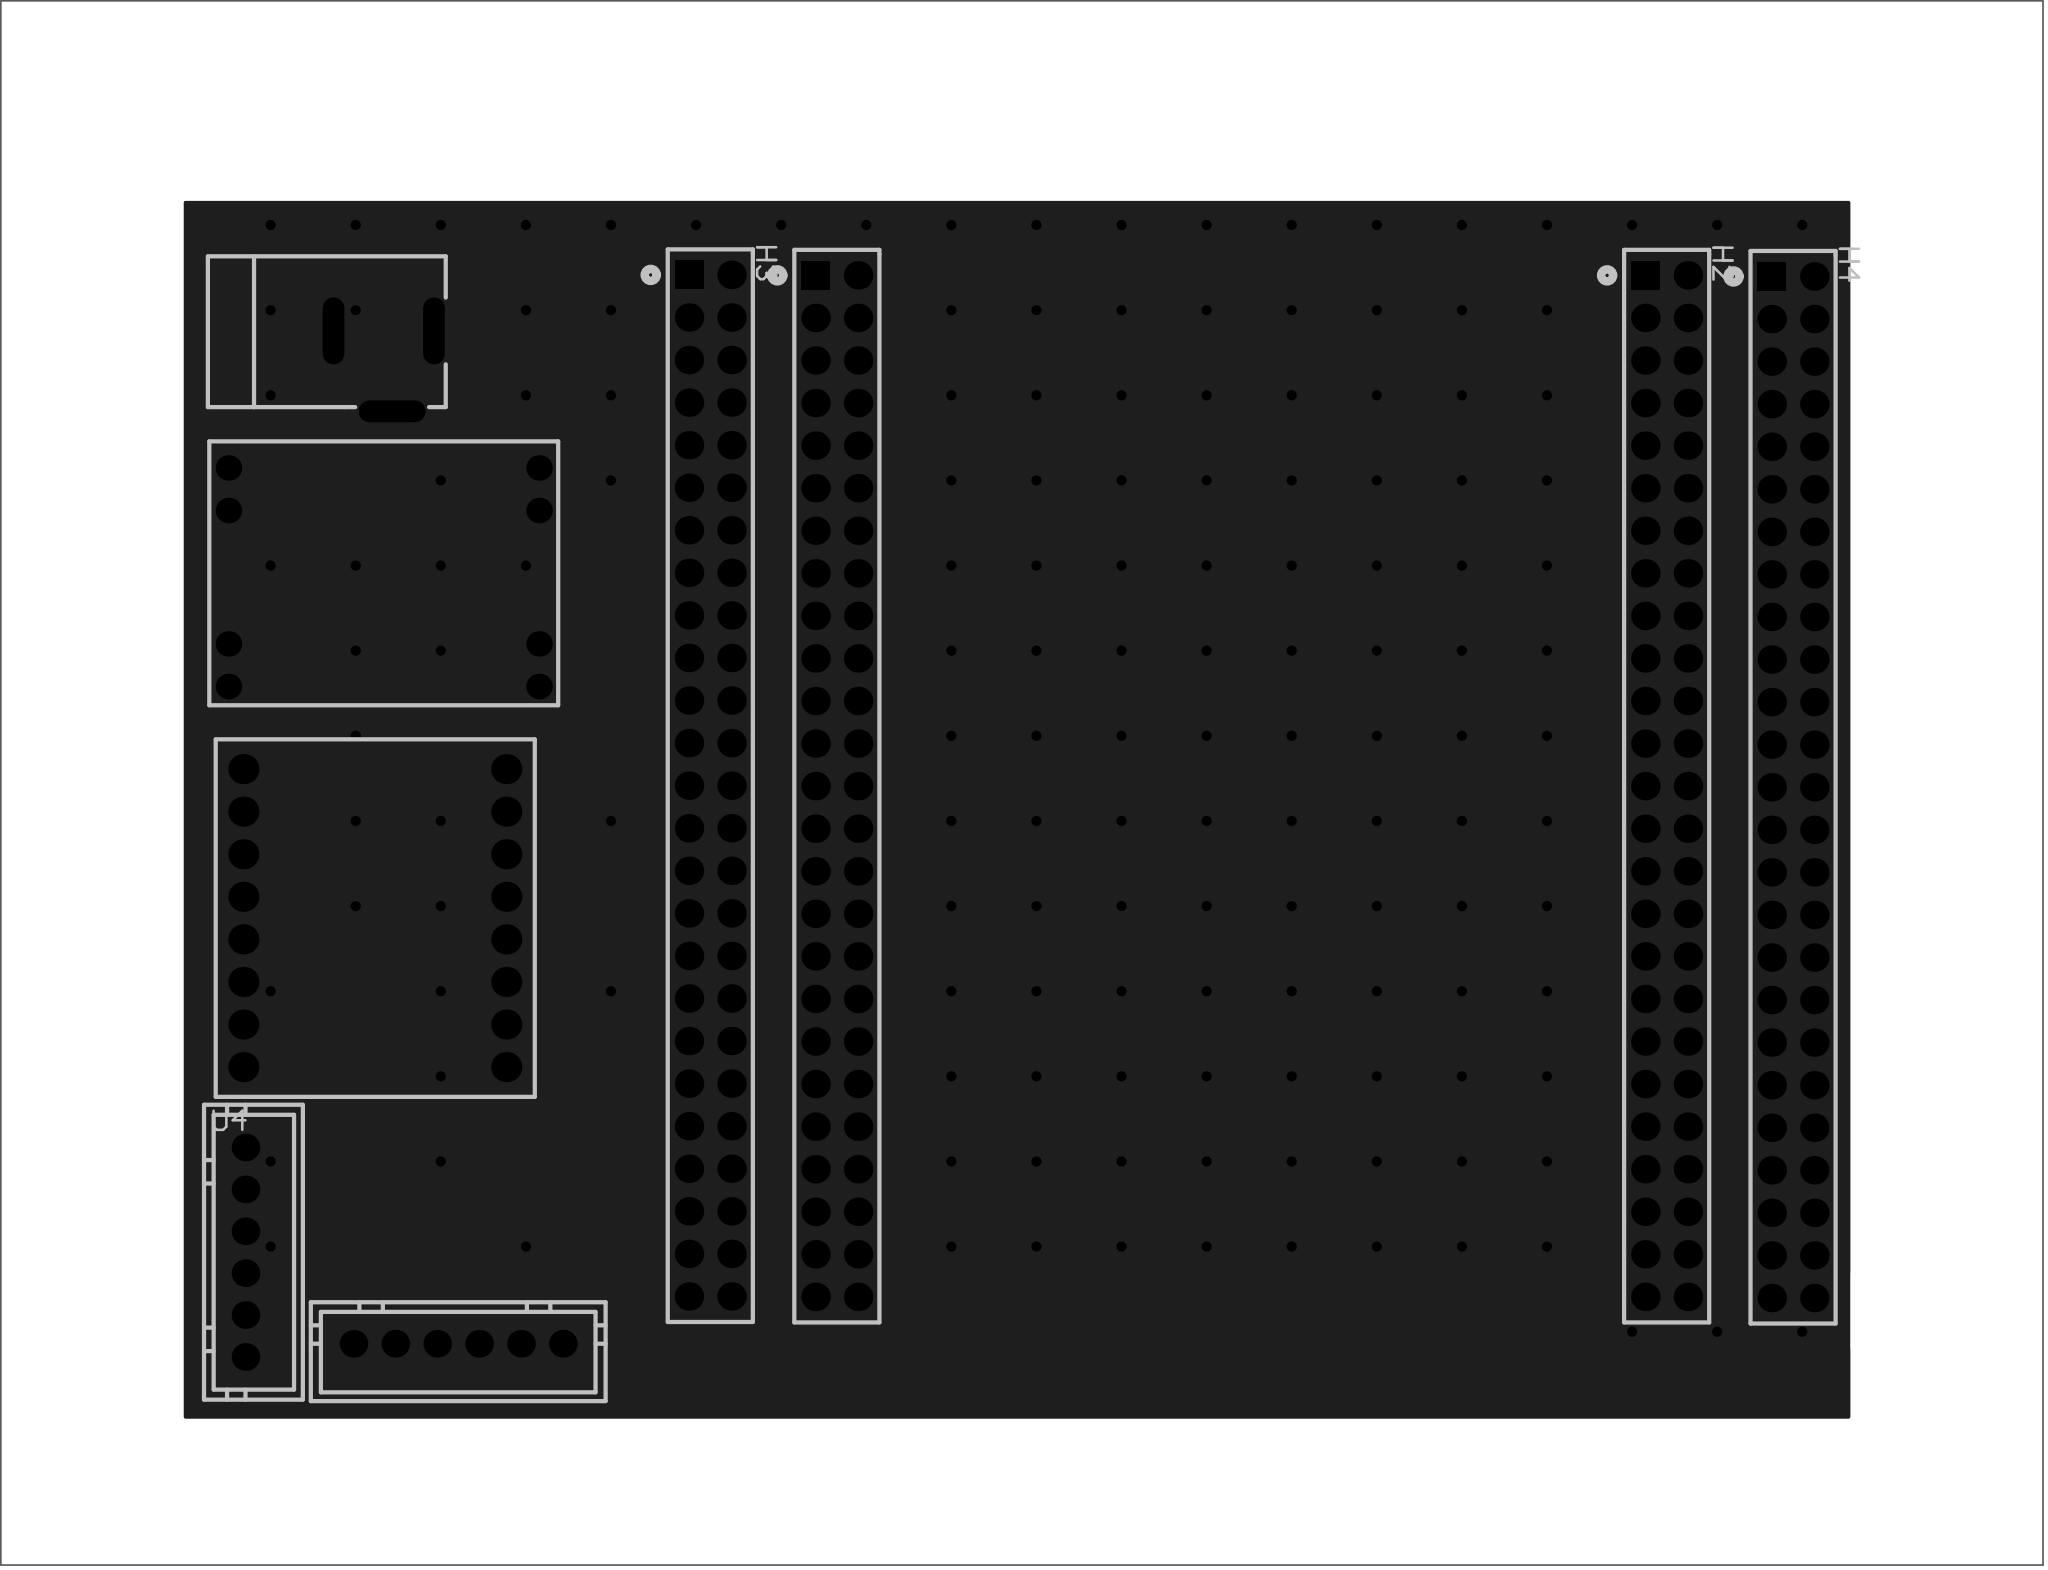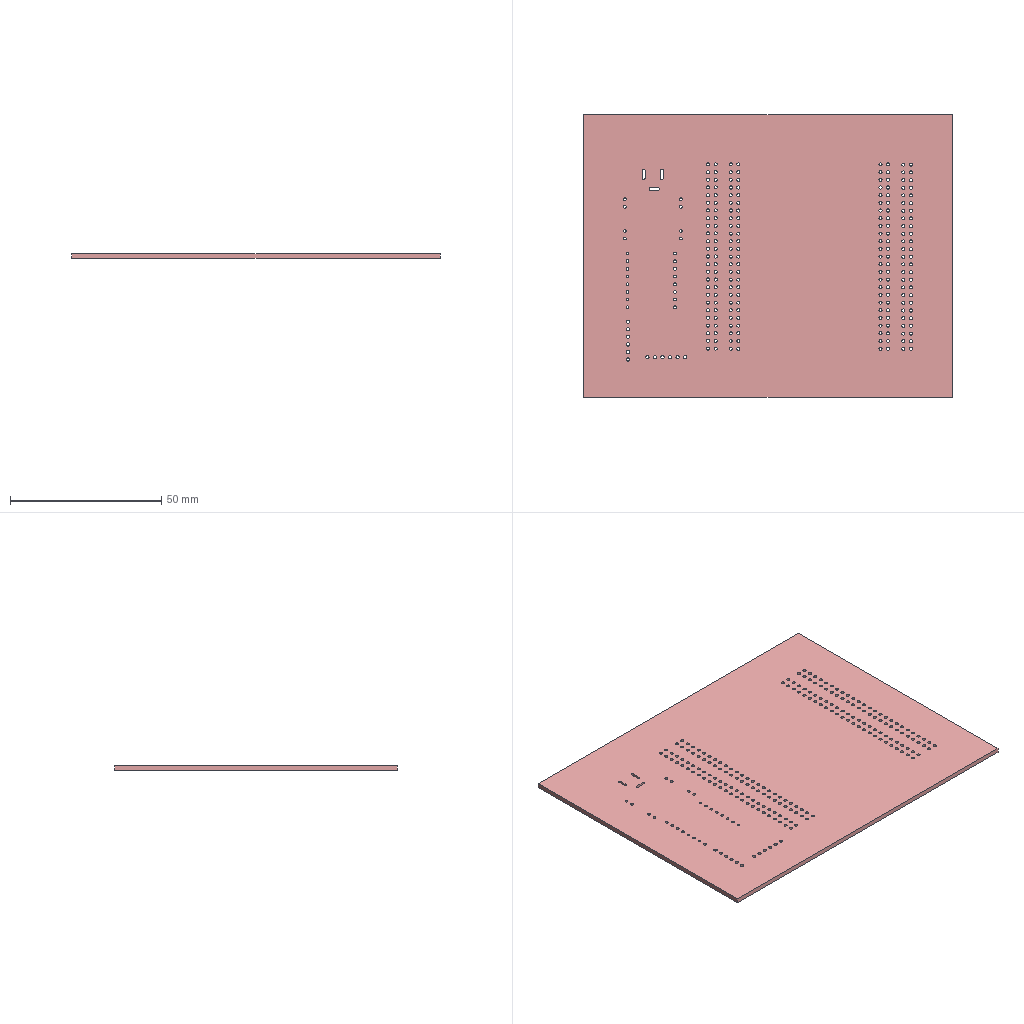Circuit board layout | Altium Designer | box 121.9 x 93.3 x 1.6 mm
Layer stack:
# Altium Designer layer stack of  (unit mm; dielectric type: 0 none, 1 core, 2 prepreg, 3 surface material)
index,name,kind,layer,copper_thickness_mm,dielectric_type,dielectric_thickness_mm,dielectric_material,dielectric_constant
0,Top Paste Mask Layer,other,,,,,,
1,Top Silkscreen Layer,other,,,,,,
2,Top Solder Mask Layer,dielectric,,,3,0.01,,3.3
3,Top Layer,copper,Top Layer,0.035,,,,
4,Dielectric1,dielectric,,,3,1.51,FR4,4.5
5,Bottom Layer,copper,Bottom Layer,0.035,,,,
6,Bottom Solder Mask Layer,dielectric,,,3,0.01,,3.3
7,Bottom Silkscreen Layer,other,,,,,,
8,Bottom Paste Mask Layer,other,,,,,,
# drill layer pairs: low layer,high layer
drill_pair,Top Layer,Bottom Layer
Part placement:
Designator,Comment,Layer,Footprint,Center-X(mm),Center-Y(mm),Rotation
DC1,,TopLayer,DC-2.0,92.71,141.097,180
H1,2.54-2*25,TopLayer,HDR-TH_50P-P2.54-V-F-R2-C25-S2.54-1,119.761,116.332,270
H2,2.54-2*25,TopLayer,HDR-TH_50P-P2.54-V-F-R2-C25-S2.54-1,169.301,116.332,270
U4,,TopLayer,tb6612,92.177,108.458,0
H3,2.54-2*25,TopLayer,HDR-TH_50P-P2.54-V-F-R2-C25-S2.54-1,112.204,116.359,270
H4,2.54-2*25,TopLayer,HDR-TH_50P-P2.54-V-F-R2-C25-S2.54-1,176.847,116.266,270
U1,XH2.54-6P through-hole,TopLayer,CONN-TH_XH2.54-6P,97.155,83.058,0
U2,XH2.54-6P through-hole,TopLayer,CONN-TH_XH2.54-6P,84.455,88.519,90
Pad and via stacks:
# Altium Designer via and pad stacks of  (unit mm). Each distinct definition once, with the count of objects using it.
# via: kind,start_layer,end_layer,hole_mm,diameter_mm,mode(0 simple;1 top-mid-bottom;2 full stack),diameter_per_layer,count,example_net
# pad: kind,layer,hole_mm,hole_type(0 round;1 square;2 slot),plating,top_size,top_shape(1 round;2 rect;3 octagon;9 rounded rect),mid_size,bottom_size,mode,footprint,size_per_layer,count,example
pad,Multi-Layer,0.8001,2,plated,4x1.3,1,4x1.3,4x1.3,0,DC-2.0,,3,DC1.2
pad,Multi-Layer,1.02,0,plated,1.7x1.7,2,1.7x1.7,1.7x1.7,0,HDR-TH_50P-P2.54-V-F-R2-C25-S2.54-1,,4,H1.1
pad,Multi-Layer,1.02,0,plated,1.7x1.7,1,1.7x1.7,1.7x1.7,0,HDR-TH_50P-P2.54-V-F-R2-C25-S2.54-1,,196,H1.2
pad,Multi-Layer,0.9,0,plated,1.8x1.8,1,1.8x1.8,1.8x1.8,0,tb6612,,16,U4.1
pad,Multi-Layer,0.9144,0,plated,1.524x1.524,1,1.524x1.524,1.524x1.524,0,,,8,1
pad,Multi-Layer,1.1,0,plated,1.65x1.65,1,1.65x1.65,1.65x1.65,0,CONN-TH_XH2.54-6P,,12,U1.1
via,Top Layer,Bottom Layer,0.3048,0.61,0,,147,GND
Copper pours:
name,layer,net,type(0 solid;1 hatched;2 none)
Top Layer-GND,Top Layer,GND,0
Bottom Layer-GND,Bottom Layer,GND,0
Design rules, without the lines most boards share:
# Altium Designer design rules of  (exported by Altium Designer, unit mm)
# columns: name | kind | enabled | priority | scope1 | scope2 | descriptor | typed fields (field=value)
copperRegion | 20 | enabled | 1 | (InNet('GND')) | All | Polygon Connect Rule(Relief Connect )(Conductor Width=10mil) (Relief Angle=90 Angle) (Entries=4) (Air Gap Width=10mil) ((InNet('GND'))),(All) | connect_style(0=relief,1=direct,2=none)=0 relief_conductor_width=0.254 relief_entries=4